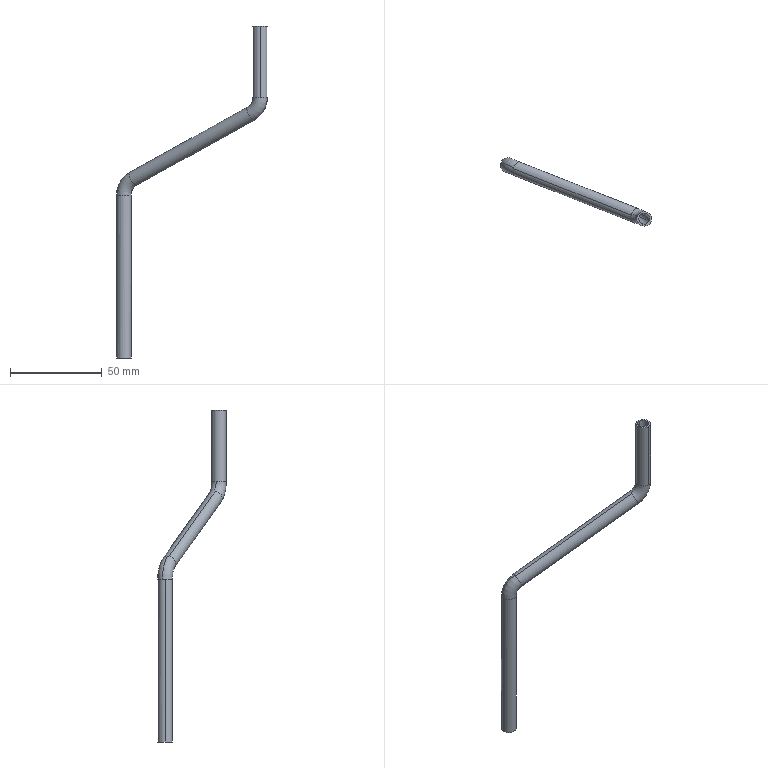Part | NX | features BREP 1 | 1 solid | 22 faces | box 82.41 x 37.379 x 181.231 mm | volume 5003 mm3 | cylinder 12 | torus 8 | plane 2 | commonest cylinder face diameters 6 x6 8 x6
STEP:
#1=CARTESIAN_POINT('',(-2.79,1.102,88.904));
#2=VERTEX_POINT('',#1);
#3=CARTESIAN_POINT('',(-3.,0.,88.904));
#4=VERTEX_POINT('',#3);
#5=CARTESIAN_POINT('',(0.,0.,88.904));
#6=DIRECTION('',(0.,0.,1.));
#7=DIRECTION('',(1.,0.,0.));
#8=AXIS2_PLACEMENT_3D('',#5,#6,#7);
#9=CIRCLE('',#8,3.);
#10=EDGE_CURVE('',#2,#4,#9,.T.);
#11=ORIENTED_EDGE('',*,*,#10,.F.);
#12=CARTESIAN_POINT('',(3.762,-1.485,100.459));
#13=VERTEX_POINT('',#12);
#14=CARTESIAN_POINT('',(9.301,-3.672,88.904));
#15=DIRECTION('',(0.3672,0.9301,0.));
#16=DIRECTION('',(-0.9301,0.3672,0.));
#17=AXIS2_PLACEMENT_3D('',#14,#15,#16);
#18=CIRCLE('',#17,13.);
#19=EDGE_CURVE('',#13,#2,#18,.F.);
#20=ORIENTED_EDGE('',*,*,#19,.F.);
#21=CARTESIAN_POINT('',(3.586,-1.99,100.417));
#22=VERTEX_POINT('',#21);
#23=CARTESIAN_POINT('',(5.04,-1.99,97.793));
#24=DIRECTION('',(0.8268,-0.3264,0.4581));
#25=DIRECTION('',(0.5312,0.1851,-0.8268));
#26=AXIS2_PLACEMENT_3D('',#23,#24,#25);
#27=CIRCLE('',#26,3.);
#28=EDGE_CURVE('',#13,#22,#27,.T.);
#29=ORIENTED_EDGE('',*,*,#28,.T.);
#30=CARTESIAN_POINT('',(6.319,-2.495,95.126));
#31=VERTEX_POINT('',#30);
#32=CARTESIAN_POINT('',(5.04,-1.99,97.793));
#33=DIRECTION('',(0.8268,-0.3264,0.4581));
#34=DIRECTION('',(0.5312,0.1851,-0.8268));
#35=AXIS2_PLACEMENT_3D('',#32,#33,#34);
#36=CIRCLE('',#35,3.);
#37=EDGE_CURVE('',#22,#31,#36,.T.);
#38=ORIENTED_EDGE('',*,*,#37,.T.);
#39=CARTESIAN_POINT('',(2.79,-1.102,88.904));
#40=VERTEX_POINT('',#39);
#41=CARTESIAN_POINT('',(9.301,-3.672,88.904));
#42=DIRECTION('',(0.3672,0.9301,0.));
#43=DIRECTION('',(-0.9301,0.3672,0.));
#44=AXIS2_PLACEMENT_3D('',#41,#42,#43);
#45=CIRCLE('',#44,7.);
#46=EDGE_CURVE('',#31,#40,#45,.F.);
#47=ORIENTED_EDGE('',*,*,#46,.T.);
#48=CARTESIAN_POINT('',(0.,0.,88.904));
#49=DIRECTION('',(0.,0.,1.));
#50=DIRECTION('',(1.,0.,0.));
#51=AXIS2_PLACEMENT_3D('',#48,#49,#50);
#52=CIRCLE('',#51,3.);
#53=EDGE_CURVE('',#4,#40,#52,.T.);
#54=ORIENTED_EDGE('',*,*,#53,.F.);
#55=EDGE_LOOP('',(#11,#20,#29,#38,#47,#54));
#56=FACE_BOUND('',#55,.T.);
#57=CARTESIAN_POINT('',(9.301,-3.672,88.904));
#58=DIRECTION('',(0.3672,0.9301,0.));
#59=DIRECTION('',(-0.9301,0.3672,0.));
#60=AXIS2_PLACEMENT_3D('',#57,#58,#59);
#61=TOROIDAL_SURFACE('',#60,10.,3.);
#62=ADVANCED_FACE('',(#56),#61,.F.);
#63=CARTESIAN_POINT('',(4.,0.,88.904));
#64=VERTEX_POINT('',#63);
#65=CARTESIAN_POINT('',(-3.721,1.469,88.904));
#66=VERTEX_POINT('',#65);
#67=CARTESIAN_POINT('',(0.,0.,88.904));
#68=DIRECTION('',(0.,0.,1.));
#69=DIRECTION('',(1.,0.,0.));
#70=AXIS2_PLACEMENT_3D('',#67,#68,#69);
#71=CIRCLE('',#70,4.);
#72=EDGE_CURVE('',#64,#66,#71,.T.);
#73=ORIENTED_EDGE('',*,*,#72,.T.);
#74=CARTESIAN_POINT('',(3.336,-1.317,101.348));
#75=VERTEX_POINT('',#74);
#76=CARTESIAN_POINT('',(9.301,-3.672,88.904));
#77=DIRECTION('',(0.3672,0.9301,0.));
#78=DIRECTION('',(-0.9301,0.3672,0.));
#79=AXIS2_PLACEMENT_3D('',#76,#77,#78);
#80=CIRCLE('',#79,14.);
#81=EDGE_CURVE('',#75,#66,#80,.F.);
#82=ORIENTED_EDGE('',*,*,#81,.F.);
#83=CARTESIAN_POINT('',(6.979,-1.99,94.294));
#84=VERTEX_POINT('',#83);
#85=CARTESIAN_POINT('',(5.04,-1.99,97.793));
#86=DIRECTION('',(0.8268,-0.3264,0.4581));
#87=DIRECTION('',(0.5312,0.1851,-0.8268));
#88=AXIS2_PLACEMENT_3D('',#85,#86,#87);
#89=CIRCLE('',#88,4.);
#90=EDGE_CURVE('',#84,#75,#89,.T.);
#91=ORIENTED_EDGE('',*,*,#90,.F.);
#92=CARTESIAN_POINT('',(6.745,-2.663,94.237));
#93=VERTEX_POINT('',#92);
#94=CARTESIAN_POINT('',(5.04,-1.99,97.793));
#95=DIRECTION('',(0.8268,-0.3264,0.4581));
#96=DIRECTION('',(0.5312,0.1851,-0.8268));
#97=AXIS2_PLACEMENT_3D('',#94,#95,#96);
#98=CIRCLE('',#97,4.);
#99=EDGE_CURVE('',#93,#84,#98,.T.);
#100=ORIENTED_EDGE('',*,*,#99,.F.);
#101=CARTESIAN_POINT('',(3.721,-1.469,88.904));
#102=VERTEX_POINT('',#101);
#103=CARTESIAN_POINT('',(9.301,-3.672,88.904));
#104=DIRECTION('',(0.3672,0.9301,0.));
#105=DIRECTION('',(-0.9301,0.3672,0.));
#106=AXIS2_PLACEMENT_3D('',#103,#104,#105);
#107=CIRCLE('',#106,6.);
#108=EDGE_CURVE('',#93,#102,#107,.F.);
#109=ORIENTED_EDGE('',*,*,#108,.T.);
#110=CARTESIAN_POINT('',(0.,0.,88.904));
#111=DIRECTION('',(0.,0.,1.));
#112=DIRECTION('',(1.,0.,0.));
#113=AXIS2_PLACEMENT_3D('',#110,#111,#112);
#114=CIRCLE('',#113,4.);
#115=EDGE_CURVE('',#102,#64,#114,.T.);
#116=ORIENTED_EDGE('',*,*,#115,.T.);
#117=EDGE_LOOP('',(#73,#82,#91,#100,#109,#116));
#118=FACE_BOUND('',#117,.T.);
#119=CARTESIAN_POINT('',(9.301,-3.672,88.904));
#120=DIRECTION('',(0.3672,0.9301,0.));
#121=DIRECTION('',(-0.9301,0.3672,0.));
#122=AXIS2_PLACEMENT_3D('',#119,#120,#121);
#123=TOROIDAL_SURFACE('',#122,10.,4.);
#124=ADVANCED_FACE('',(#118),#123,.T.);
#125=CARTESIAN_POINT('',(70.649,-27.893,130.772));
#126=VERTEX_POINT('',#125);
#127=CARTESIAN_POINT('',(70.824,-27.389,130.814));
#128=VERTEX_POINT('',#127);
#129=CARTESIAN_POINT('',(69.37,-27.389,133.438));
#130=DIRECTION('',(0.8268,-0.3264,0.4581));
#131=DIRECTION('',(0.5312,0.1851,-0.8268));
#132=AXIS2_PLACEMENT_3D('',#129,#130,#131);
#133=CIRCLE('',#132,3.);
#134=EDGE_CURVE('',#126,#128,#133,.T.);
#135=ORIENTED_EDGE('',*,*,#134,.F.);
#136=CARTESIAN_POINT('',(77.201,-30.48,142.327));
#137=VERTEX_POINT('',#136);
#138=CARTESIAN_POINT('',(65.109,-25.706,142.327));
#139=DIRECTION('',(-0.3672,-0.9301,0.));
#140=DIRECTION('',(0.9301,-0.3672,0.));
#141=AXIS2_PLACEMENT_3D('',#138,#139,#140);
#142=CIRCLE('',#141,13.);
#143=EDGE_CURVE('',#126,#137,#142,.T.);
#144=ORIENTED_EDGE('',*,*,#143,.T.);
#145=CARTESIAN_POINT('',(74.41,-26.379,142.327));
#146=VERTEX_POINT('',#145);
#147=CARTESIAN_POINT('',(74.41,-29.379,142.327));
#148=DIRECTION('',(0.,0.,1.));
#149=DIRECTION('',(1.,0.,0.));
#150=AXIS2_PLACEMENT_3D('',#147,#148,#149);
#151=CIRCLE('',#150,3.);
#152=EDGE_CURVE('',#137,#146,#151,.T.);
#153=ORIENTED_EDGE('',*,*,#152,.T.);
#154=CARTESIAN_POINT('',(71.62,-28.277,142.327));
#155=VERTEX_POINT('',#154);
#156=CARTESIAN_POINT('',(74.41,-29.379,142.327));
#157=DIRECTION('',(0.,0.,1.));
#158=DIRECTION('',(1.,0.,0.));
#159=AXIS2_PLACEMENT_3D('',#156,#157,#158);
#160=CIRCLE('',#159,3.);
#161=EDGE_CURVE('',#146,#155,#160,.T.);
#162=ORIENTED_EDGE('',*,*,#161,.T.);
#163=CARTESIAN_POINT('',(68.092,-26.884,136.105));
#164=VERTEX_POINT('',#163);
#165=CARTESIAN_POINT('',(65.109,-25.706,142.327));
#166=DIRECTION('',(-0.3672,-0.9301,0.));
#167=DIRECTION('',(0.9301,-0.3672,0.));
#168=AXIS2_PLACEMENT_3D('',#165,#166,#167);
#169=CIRCLE('',#168,7.);
#170=EDGE_CURVE('',#164,#155,#169,.T.);
#171=ORIENTED_EDGE('',*,*,#170,.F.);
#172=CARTESIAN_POINT('',(69.37,-27.389,133.438));
#173=DIRECTION('',(0.8268,-0.3264,0.4581));
#174=DIRECTION('',(0.5312,0.1851,-0.8268));
#175=AXIS2_PLACEMENT_3D('',#172,#173,#174);
#176=CIRCLE('',#175,3.);
#177=EDGE_CURVE('',#128,#164,#176,.T.);
#178=ORIENTED_EDGE('',*,*,#177,.F.);
#179=EDGE_LOOP('',(#135,#144,#153,#162,#171,#178));
#180=FACE_BOUND('',#179,.T.);
#181=CARTESIAN_POINT('',(65.109,-25.706,142.327));
#182=DIRECTION('',(-0.3672,-0.9301,0.));
#183=DIRECTION('',(0.9301,-0.3672,0.));
#184=AXIS2_PLACEMENT_3D('',#181,#182,#183);
#185=TOROIDAL_SURFACE('',#184,10.,3.);
#186=ADVANCED_FACE('',(#180),#185,.F.);
#187=CARTESIAN_POINT('',(67.432,-27.389,136.937));
#188=VERTEX_POINT('',#187);
#189=CARTESIAN_POINT('',(71.075,-28.062,129.883));
#190=VERTEX_POINT('',#189);
#191=CARTESIAN_POINT('',(69.37,-27.389,133.438));
#192=DIRECTION('',(0.8268,-0.3264,0.4581));
#193=DIRECTION('',(0.5312,0.1851,-0.8268));
#194=AXIS2_PLACEMENT_3D('',#191,#192,#193);
#195=CIRCLE('',#194,4.);
#196=EDGE_CURVE('',#188,#190,#195,.T.);
#197=ORIENTED_EDGE('',*,*,#196,.T.);
#198=CARTESIAN_POINT('',(78.131,-30.847,142.327));
#199=VERTEX_POINT('',#198);
#200=CARTESIAN_POINT('',(65.109,-25.706,142.327));
#201=DIRECTION('',(-0.3672,-0.9301,0.));
#202=DIRECTION('',(0.9301,-0.3672,0.));
#203=AXIS2_PLACEMENT_3D('',#200,#201,#202);
#204=CIRCLE('',#203,14.);
#205=EDGE_CURVE('',#190,#199,#204,.T.);
#206=ORIENTED_EDGE('',*,*,#205,.T.);
#207=CARTESIAN_POINT('',(74.41,-33.379,142.327));
#208=VERTEX_POINT('',#207);
#209=CARTESIAN_POINT('',(74.41,-29.379,142.327));
#210=DIRECTION('',(0.,0.,1.));
#211=DIRECTION('',(1.,0.,0.));
#212=AXIS2_PLACEMENT_3D('',#209,#210,#211);
#213=CIRCLE('',#212,4.);
#214=EDGE_CURVE('',#208,#199,#213,.T.);
#215=ORIENTED_EDGE('',*,*,#214,.F.);
#216=CARTESIAN_POINT('',(70.69,-27.91,142.327));
#217=VERTEX_POINT('',#216);
#218=CARTESIAN_POINT('',(74.41,-29.379,142.327));
#219=DIRECTION('',(0.,0.,1.));
#220=DIRECTION('',(1.,0.,0.));
#221=AXIS2_PLACEMENT_3D('',#218,#219,#220);
#222=CIRCLE('',#221,4.);
#223=EDGE_CURVE('',#217,#208,#222,.T.);
#224=ORIENTED_EDGE('',*,*,#223,.F.);
#225=CARTESIAN_POINT('',(67.666,-26.716,136.994));
#226=VERTEX_POINT('',#225);
#227=CARTESIAN_POINT('',(65.109,-25.706,142.327));
#228=DIRECTION('',(-0.3672,-0.9301,0.));
#229=DIRECTION('',(0.9301,-0.3672,0.));
#230=AXIS2_PLACEMENT_3D('',#227,#228,#229);
#231=CIRCLE('',#230,6.);
#232=EDGE_CURVE('',#226,#217,#231,.T.);
#233=ORIENTED_EDGE('',*,*,#232,.F.);
#234=CARTESIAN_POINT('',(69.37,-27.389,133.438));
#235=DIRECTION('',(0.8268,-0.3264,0.4581));
#236=DIRECTION('',(0.5312,0.1851,-0.8268));
#237=AXIS2_PLACEMENT_3D('',#234,#235,#236);
#238=CIRCLE('',#237,4.);
#239=EDGE_CURVE('',#226,#188,#238,.T.);
#240=ORIENTED_EDGE('',*,*,#239,.T.);
#241=EDGE_LOOP('',(#197,#206,#215,#224,#233,#240));
#242=FACE_BOUND('',#241,.T.);
#243=CARTESIAN_POINT('',(65.109,-25.706,142.327));
#244=DIRECTION('',(-0.3672,-0.9301,0.));
#245=DIRECTION('',(0.9301,-0.3672,0.));
#246=AXIS2_PLACEMENT_3D('',#243,#244,#245);
#247=TOROIDAL_SURFACE('',#246,10.,4.);
#248=ADVANCED_FACE('',(#242),#247,.T.);
#249=ORIENTED_EDGE('',*,*,#72,.F.);
#250=CARTESIAN_POINT('',(4.,0.,0.));
#251=VERTEX_POINT('',#250);
#252=CARTESIAN_POINT('',(4.,0.,88.904));
#253=DIRECTION('',(0.,0.,-1.));
#254=VECTOR('',#253,1000.);
#255=LINE('',#252,#254);
#256=EDGE_CURVE('',#64,#251,#255,.T.);
#257=ORIENTED_EDGE('',*,*,#256,.T.);
#258=CARTESIAN_POINT('',(-4.,0.,0.));
#259=VERTEX_POINT('',#258);
#260=CARTESIAN_POINT('',(0.,0.,0.));
#261=DIRECTION('',(0.,0.,1.));
#262=DIRECTION('',(1.,0.,0.));
#263=AXIS2_PLACEMENT_3D('',#260,#261,#262);
#264=CIRCLE('',#263,4.);
#265=EDGE_CURVE('',#251,#259,#264,.T.);
#266=ORIENTED_EDGE('',*,*,#265,.T.);
#267=CARTESIAN_POINT('',(-4.,0.,88.904));
#268=VERTEX_POINT('',#267);
#269=CARTESIAN_POINT('',(-4.,0.,88.904));
#270=DIRECTION('',(0.,0.,-1.));
#271=VECTOR('',#270,1000.);
#272=LINE('',#269,#271);
#273=EDGE_CURVE('',#268,#259,#272,.T.);
#274=ORIENTED_EDGE('',*,*,#273,.F.);
#275=CARTESIAN_POINT('',(0.,0.,88.904));
#276=DIRECTION('',(0.,0.,1.));
#277=DIRECTION('',(1.,0.,0.));
#278=AXIS2_PLACEMENT_3D('',#275,#276,#277);
#279=CIRCLE('',#278,4.);
#280=EDGE_CURVE('',#66,#268,#279,.T.);
#281=ORIENTED_EDGE('',*,*,#280,.F.);
#282=EDGE_LOOP('',(#249,#257,#266,#274,#281));
#283=FACE_BOUND('',#282,.T.);
#284=CARTESIAN_POINT('',(0.,0.,88.904));
#285=DIRECTION('',(0.,0.,-1.));
#286=DIRECTION('',(-1.,0.,0.));
#287=AXIS2_PLACEMENT_3D('',#284,#285,#286);
#288=CYLINDRICAL_SURFACE('',#287,4.);
#289=ADVANCED_FACE('',(#283),#288,.T.);
#290=ORIENTED_EDGE('',*,*,#53,.T.);
#291=CARTESIAN_POINT('',(3.,0.,88.904));
#292=VERTEX_POINT('',#291);
#293=CARTESIAN_POINT('',(0.,0.,88.904));
#294=DIRECTION('',(0.,0.,1.));
#295=DIRECTION('',(1.,0.,0.));
#296=AXIS2_PLACEMENT_3D('',#293,#294,#295);
#297=CIRCLE('',#296,3.);
#298=EDGE_CURVE('',#40,#292,#297,.T.);
#299=ORIENTED_EDGE('',*,*,#298,.T.);
#300=CARTESIAN_POINT('',(3.,0.,0.));
#301=VERTEX_POINT('',#300);
#302=CARTESIAN_POINT('',(3.,0.,88.904));
#303=DIRECTION('',(0.,0.,-1.));
#304=VECTOR('',#303,1000.);
#305=LINE('',#302,#304);
#306=EDGE_CURVE('',#292,#301,#305,.T.);
#307=ORIENTED_EDGE('',*,*,#306,.T.);
#308=CARTESIAN_POINT('',(-3.,0.,0.));
#309=VERTEX_POINT('',#308);
#310=CARTESIAN_POINT('',(0.,0.,0.));
#311=DIRECTION('',(0.,0.,1.));
#312=DIRECTION('',(1.,0.,0.));
#313=AXIS2_PLACEMENT_3D('',#310,#311,#312);
#314=CIRCLE('',#313,3.);
#315=EDGE_CURVE('',#309,#301,#314,.T.);
#316=ORIENTED_EDGE('',*,*,#315,.F.);
#317=CARTESIAN_POINT('',(-3.,0.,88.904));
#318=DIRECTION('',(0.,0.,-1.));
#319=VECTOR('',#318,1000.);
#320=LINE('',#317,#319);
#321=EDGE_CURVE('',#4,#309,#320,.T.);
#322=ORIENTED_EDGE('',*,*,#321,.F.);
#323=EDGE_LOOP('',(#290,#299,#307,#316,#322));
#324=FACE_BOUND('',#323,.T.);
#325=CARTESIAN_POINT('',(0.,0.,88.904));
#326=DIRECTION('',(0.,0.,-1.));
#327=DIRECTION('',(-1.,0.,0.));
#328=AXIS2_PLACEMENT_3D('',#325,#326,#327);
#329=CYLINDRICAL_SURFACE('',#328,3.);
#330=ADVANCED_FACE('',(#324),#329,.F.);
#331=ORIENTED_EDGE('',*,*,#37,.F.);
#332=CARTESIAN_POINT('',(67.916,-27.389,136.062));
#333=VERTEX_POINT('',#332);
#334=CARTESIAN_POINT('',(3.586,-1.99,100.417));
#335=DIRECTION('',(0.8268,-0.3264,0.4581));
#336=VECTOR('',#335,1000.);
#337=LINE('',#334,#336);
#338=EDGE_CURVE('',#333,#22,#337,.F.);
#339=ORIENTED_EDGE('',*,*,#338,.F.);
#340=CARTESIAN_POINT('',(69.37,-27.389,133.438));
#341=DIRECTION('',(0.8268,-0.3264,0.4581));
#342=DIRECTION('',(0.5312,0.1851,-0.8268));
#343=AXIS2_PLACEMENT_3D('',#340,#341,#342);
#344=CIRCLE('',#343,3.);
#345=EDGE_CURVE('',#333,#126,#344,.T.);
#346=ORIENTED_EDGE('',*,*,#345,.T.);
#347=ORIENTED_EDGE('',*,*,#134,.T.);
#348=CARTESIAN_POINT('',(6.494,-1.99,95.169));
#349=VERTEX_POINT('',#348);
#350=CARTESIAN_POINT('',(6.494,-1.99,95.169));
#351=DIRECTION('',(0.8268,-0.3264,0.4581));
#352=VECTOR('',#351,1000.);
#353=LINE('',#350,#352);
#354=EDGE_CURVE('',#128,#349,#353,.F.);
#355=ORIENTED_EDGE('',*,*,#354,.T.);
#356=CARTESIAN_POINT('',(5.04,-1.99,97.793));
#357=DIRECTION('',(0.8268,-0.3264,0.4581));
#358=DIRECTION('',(0.5312,0.1851,-0.8268));
#359=AXIS2_PLACEMENT_3D('',#356,#357,#358);
#360=CIRCLE('',#359,3.);
#361=EDGE_CURVE('',#31,#349,#360,.T.);
#362=ORIENTED_EDGE('',*,*,#361,.F.);
#363=EDGE_LOOP('',(#331,#339,#346,#347,#355,#362));
#364=FACE_BOUND('',#363,.T.);
#365=CARTESIAN_POINT('',(5.04,-1.99,97.793));
#366=DIRECTION('',(0.8268,-0.3264,0.4581));
#367=DIRECTION('',(0.4847,0.,-0.8747));
#368=AXIS2_PLACEMENT_3D('',#365,#366,#367);
#369=CYLINDRICAL_SURFACE('',#368,3.);
#370=ADVANCED_FACE('',(#364),#369,.F.);
#371=ORIENTED_EDGE('',*,*,#90,.T.);
#372=CARTESIAN_POINT('',(3.101,-1.99,101.292));
#373=VERTEX_POINT('',#372);
#374=CARTESIAN_POINT('',(5.04,-1.99,97.793));
#375=DIRECTION('',(0.8268,-0.3264,0.4581));
#376=DIRECTION('',(0.5312,0.1851,-0.8268));
#377=AXIS2_PLACEMENT_3D('',#374,#375,#376);
#378=CIRCLE('',#377,4.);
#379=EDGE_CURVE('',#75,#373,#378,.T.);
#380=ORIENTED_EDGE('',*,*,#379,.T.);
#381=CARTESIAN_POINT('',(3.101,-1.99,101.292));
#382=DIRECTION('',(0.8268,-0.3264,0.4581));
#383=VECTOR('',#382,1000.);
#384=LINE('',#381,#383);
#385=EDGE_CURVE('',#188,#373,#384,.F.);
#386=ORIENTED_EDGE('',*,*,#385,.F.);
#387=ORIENTED_EDGE('',*,*,#239,.F.);
#388=CARTESIAN_POINT('',(71.309,-27.389,129.94));
#389=VERTEX_POINT('',#388);
#390=CARTESIAN_POINT('',(69.37,-27.389,133.438));
#391=DIRECTION('',(0.8268,-0.3264,0.4581));
#392=DIRECTION('',(0.5312,0.1851,-0.8268));
#393=AXIS2_PLACEMENT_3D('',#390,#391,#392);
#394=CIRCLE('',#393,4.);
#395=EDGE_CURVE('',#389,#226,#394,.T.);
#396=ORIENTED_EDGE('',*,*,#395,.F.);
#397=CARTESIAN_POINT('',(6.979,-1.99,94.294));
#398=DIRECTION('',(0.8268,-0.3264,0.4581));
#399=VECTOR('',#398,1000.);
#400=LINE('',#397,#399);
#401=EDGE_CURVE('',#389,#84,#400,.F.);
#402=ORIENTED_EDGE('',*,*,#401,.T.);
#403=EDGE_LOOP('',(#371,#380,#386,#387,#396,#402));
#404=FACE_BOUND('',#403,.T.);
#405=CARTESIAN_POINT('',(5.04,-1.99,97.793));
#406=DIRECTION('',(0.8268,-0.3264,0.4581));
#407=DIRECTION('',(0.4847,0.,-0.8747));
#408=AXIS2_PLACEMENT_3D('',#405,#406,#407);
#409=CYLINDRICAL_SURFACE('',#408,4.);
#410=ADVANCED_FACE('',(#404),#409,.T.);
#411=ORIENTED_EDGE('',*,*,#161,.F.);
#412=CARTESIAN_POINT('',(74.41,-26.379,181.231));
#413=VERTEX_POINT('',#412);
#414=CARTESIAN_POINT('',(74.41,-26.379,142.327));
#415=DIRECTION('',(0.,0.,1.));
#416=VECTOR('',#415,1000.);
#417=LINE('',#414,#416);
#418=EDGE_CURVE('',#146,#413,#417,.T.);
#419=ORIENTED_EDGE('',*,*,#418,.T.);
#420=CARTESIAN_POINT('',(74.41,-32.379,181.231));
#421=VERTEX_POINT('',#420);
#422=CARTESIAN_POINT('',(74.41,-29.379,181.231));
#423=DIRECTION('',(0.,0.,1.));
#424=DIRECTION('',(1.,0.,0.));
#425=AXIS2_PLACEMENT_3D('',#422,#423,#424);
#426=CIRCLE('',#425,3.);
#427=EDGE_CURVE('',#413,#421,#426,.T.);
#428=ORIENTED_EDGE('',*,*,#427,.T.);
#429=CARTESIAN_POINT('',(74.41,-32.379,142.327));
#430=VERTEX_POINT('',#429);
#431=CARTESIAN_POINT('',(74.41,-32.379,142.327));
#432=DIRECTION('',(0.,0.,1.));
#433=VECTOR('',#432,1000.);
#434=LINE('',#431,#433);
#435=EDGE_CURVE('',#430,#421,#434,.T.);
#436=ORIENTED_EDGE('',*,*,#435,.F.);
#437=CARTESIAN_POINT('',(74.41,-29.379,142.327));
#438=DIRECTION('',(0.,0.,1.));
#439=DIRECTION('',(1.,0.,0.));
#440=AXIS2_PLACEMENT_3D('',#437,#438,#439);
#441=CIRCLE('',#440,3.);
#442=EDGE_CURVE('',#155,#430,#441,.T.);
#443=ORIENTED_EDGE('',*,*,#442,.F.);
#444=EDGE_LOOP('',(#411,#419,#428,#436,#443));
#445=FACE_BOUND('',#444,.T.);
#446=CARTESIAN_POINT('',(74.41,-29.379,142.327));
#447=DIRECTION('',(0.,0.,1.));
#448=DIRECTION('',(0.,-1.,0.));
#449=AXIS2_PLACEMENT_3D('',#446,#447,#448);
#450=CYLINDRICAL_SURFACE('',#449,3.);
#451=ADVANCED_FACE('',(#445),#450,.F.);
#452=ORIENTED_EDGE('',*,*,#214,.T.);
#453=CARTESIAN_POINT('',(74.41,-25.379,142.327));
#454=VERTEX_POINT('',#453);
#455=CARTESIAN_POINT('',(74.41,-29.379,142.327));
#456=DIRECTION('',(0.,0.,1.));
#457=DIRECTION('',(1.,0.,0.));
#458=AXIS2_PLACEMENT_3D('',#455,#456,#457);
#459=CIRCLE('',#458,4.);
#460=EDGE_CURVE('',#199,#454,#459,.T.);
#461=ORIENTED_EDGE('',*,*,#460,.T.);
#462=CARTESIAN_POINT('',(74.41,-25.379,181.231));
#463=VERTEX_POINT('',#462);
#464=CARTESIAN_POINT('',(74.41,-25.379,142.327));
#465=DIRECTION('',(0.,0.,1.));
#466=VECTOR('',#465,1000.);
#467=LINE('',#464,#466);
#468=EDGE_CURVE('',#454,#463,#467,.T.);
#469=ORIENTED_EDGE('',*,*,#468,.T.);
#470=CARTESIAN_POINT('',(74.41,-33.379,181.231));
#471=VERTEX_POINT('',#470);
#472=CARTESIAN_POINT('',(74.41,-29.379,181.231));
#473=DIRECTION('',(0.,0.,1.));
#474=DIRECTION('',(1.,0.,0.));
#475=AXIS2_PLACEMENT_3D('',#472,#473,#474);
#476=CIRCLE('',#475,4.);
#477=EDGE_CURVE('',#471,#463,#476,.T.);
#478=ORIENTED_EDGE('',*,*,#477,.F.);
#479=CARTESIAN_POINT('',(74.41,-33.379,142.327));
#480=DIRECTION('',(0.,0.,1.));
#481=VECTOR('',#480,1000.);
#482=LINE('',#479,#481);
#483=EDGE_CURVE('',#208,#471,#482,.T.);
#484=ORIENTED_EDGE('',*,*,#483,.F.);
#485=EDGE_LOOP('',(#452,#461,#469,#478,#484));
#486=FACE_BOUND('',#485,.T.);
#487=CARTESIAN_POINT('',(74.41,-29.379,142.327));
#488=DIRECTION('',(0.,0.,1.));
#489=DIRECTION('',(0.,-1.,0.));
#490=AXIS2_PLACEMENT_3D('',#487,#488,#489);
#491=CYLINDRICAL_SURFACE('',#490,4.);
#492=ADVANCED_FACE('',(#486),#491,.T.);
#493=ORIENTED_EDGE('',*,*,#468,.F.);
#494=CARTESIAN_POINT('',(74.41,-29.379,142.327));
#495=DIRECTION('',(0.,0.,1.));
#496=DIRECTION('',(1.,0.,0.));
#497=AXIS2_PLACEMENT_3D('',#494,#495,#496);
#498=CIRCLE('',#497,4.);
#499=EDGE_CURVE('',#454,#217,#498,.T.);
#500=ORIENTED_EDGE('',*,*,#499,.T.);
#501=ORIENTED_EDGE('',*,*,#223,.T.);
#502=ORIENTED_EDGE('',*,*,#483,.T.);
#503=CARTESIAN_POINT('',(74.41,-29.379,181.231));
#504=DIRECTION('',(0.,0.,1.));
#505=DIRECTION('',(1.,0.,0.));
#506=AXIS2_PLACEMENT_3D('',#503,#504,#505);
#507=CIRCLE('',#506,4.);
#508=EDGE_CURVE('',#463,#471,#507,.T.);
#509=ORIENTED_EDGE('',*,*,#508,.F.);
#510=EDGE_LOOP('',(#493,#500,#501,#502,#509));
#511=FACE_BOUND('',#510,.T.);
#512=CARTESIAN_POINT('',(74.41,-29.379,142.327));
#513=DIRECTION('',(0.,0.,1.));
#514=DIRECTION('',(0.,-1.,0.));
#515=AXIS2_PLACEMENT_3D('',#512,#513,#514);
#516=CYLINDRICAL_SURFACE('',#515,4.);
#517=ADVANCED_FACE('',(#511),#516,.T.);
#518=ORIENTED_EDGE('',*,*,#418,.F.);
#519=ORIENTED_EDGE('',*,*,#152,.F.);
#520=CARTESIAN_POINT('',(74.41,-29.379,142.327));
#521=DIRECTION('',(0.,0.,1.));
#522=DIRECTION('',(1.,0.,0.));
#523=AXIS2_PLACEMENT_3D('',#520,#521,#522);
#524=CIRCLE('',#523,3.);
#525=EDGE_CURVE('',#430,#137,#524,.T.);
#526=ORIENTED_EDGE('',*,*,#525,.F.);
#527=ORIENTED_EDGE('',*,*,#435,.T.);
#528=CARTESIAN_POINT('',(74.41,-29.379,181.231));
#529=DIRECTION('',(0.,0.,1.));
#530=DIRECTION('',(1.,0.,0.));
#531=AXIS2_PLACEMENT_3D('',#528,#529,#530);
#532=CIRCLE('',#531,3.);
#533=EDGE_CURVE('',#421,#413,#532,.T.);
#534=ORIENTED_EDGE('',*,*,#533,.T.);
#535=EDGE_LOOP('',(#518,#519,#526,#527,#534));
#536=FACE_BOUND('',#535,.T.);
#537=CARTESIAN_POINT('',(74.41,-29.379,142.327));
#538=DIRECTION('',(0.,0.,1.));
#539=DIRECTION('',(0.,-1.,0.));
#540=AXIS2_PLACEMENT_3D('',#537,#538,#539);
#541=CYLINDRICAL_SURFACE('',#540,3.);
#542=ADVANCED_FACE('',(#536),#541,.F.);
#543=ORIENTED_EDGE('',*,*,#205,.F.);
#544=CARTESIAN_POINT('',(69.37,-27.389,133.438));
#545=DIRECTION('',(0.8268,-0.3264,0.4581));
#546=DIRECTION('',(0.5312,0.1851,-0.8268));
#547=AXIS2_PLACEMENT_3D('',#544,#545,#546);
#548=CIRCLE('',#547,4.);
#549=EDGE_CURVE('',#190,#389,#548,.T.);
#550=ORIENTED_EDGE('',*,*,#549,.T.);
#551=ORIENTED_EDGE('',*,*,#395,.T.);
#552=ORIENTED_EDGE('',*,*,#232,.T.);
#553=ORIENTED_EDGE('',*,*,#499,.F.);
#554=ORIENTED_EDGE('',*,*,#460,.F.);
#555=EDGE_LOOP('',(#543,#550,#551,#552,#553,#554));
#556=FACE_BOUND('',#555,.T.);
#557=CARTESIAN_POINT('',(65.109,-25.706,142.327));
#558=DIRECTION('',(-0.3672,-0.9301,0.));
#559=DIRECTION('',(0.9301,-0.3672,0.));
#560=AXIS2_PLACEMENT_3D('',#557,#558,#559);
#561=TOROIDAL_SURFACE('',#560,10.,4.);
#562=ADVANCED_FACE('',(#556),#561,.T.);
#563=ORIENTED_EDGE('',*,*,#143,.F.);
#564=ORIENTED_EDGE('',*,*,#345,.F.);
#565=CARTESIAN_POINT('',(69.37,-27.389,133.438));
#566=DIRECTION('',(0.8268,-0.3264,0.4581));
#567=DIRECTION('',(0.5312,0.1851,-0.8268));
#568=AXIS2_PLACEMENT_3D('',#565,#566,#567);
#569=CIRCLE('',#568,3.);
#570=EDGE_CURVE('',#164,#333,#569,.T.);
#571=ORIENTED_EDGE('',*,*,#570,.F.);
#572=ORIENTED_EDGE('',*,*,#170,.T.);
#573=ORIENTED_EDGE('',*,*,#442,.T.);
#574=ORIENTED_EDGE('',*,*,#525,.T.);
#575=EDGE_LOOP('',(#563,#564,#571,#572,#573,#574));
#576=FACE_BOUND('',#575,.T.);
#577=CARTESIAN_POINT('',(65.109,-25.706,142.327));
#578=DIRECTION('',(-0.3672,-0.9301,0.));
#579=DIRECTION('',(0.9301,-0.3672,0.));
#580=AXIS2_PLACEMENT_3D('',#577,#578,#579);
#581=TOROIDAL_SURFACE('',#580,10.,3.);
#582=ADVANCED_FACE('',(#576),#581,.F.);
#583=ORIENTED_EDGE('',*,*,#385,.T.);
#584=CARTESIAN_POINT('',(5.04,-1.99,97.793));
#585=DIRECTION('',(0.8268,-0.3264,0.4581));
#586=DIRECTION('',(0.5312,0.1851,-0.8268));
#587=AXIS2_PLACEMENT_3D('',#584,#585,#586);
#588=CIRCLE('',#587,4.);
#589=EDGE_CURVE('',#373,#93,#588,.T.);
#590=ORIENTED_EDGE('',*,*,#589,.T.);
#591=ORIENTED_EDGE('',*,*,#99,.T.);
#592=ORIENTED_EDGE('',*,*,#401,.F.);
#593=ORIENTED_EDGE('',*,*,#549,.F.);
#594=ORIENTED_EDGE('',*,*,#196,.F.);
#595=EDGE_LOOP('',(#583,#590,#591,#592,#593,#594));
#596=FACE_BOUND('',#595,.T.);
#597=CARTESIAN_POINT('',(5.04,-1.99,97.793));
#598=DIRECTION('',(0.8268,-0.3264,0.4581));
#599=DIRECTION('',(0.4847,0.,-0.8747));
#600=AXIS2_PLACEMENT_3D('',#597,#598,#599);
#601=CYLINDRICAL_SURFACE('',#600,4.);
#602=ADVANCED_FACE('',(#596),#601,.T.);
#603=ORIENTED_EDGE('',*,*,#338,.T.);
#604=ORIENTED_EDGE('',*,*,#28,.F.);
#605=CARTESIAN_POINT('',(5.04,-1.99,97.793));
#606=DIRECTION('',(0.8268,-0.3264,0.4581));
#607=DIRECTION('',(0.5312,0.1851,-0.8268));
#608=AXIS2_PLACEMENT_3D('',#605,#606,#607);
#609=CIRCLE('',#608,3.);
#610=EDGE_CURVE('',#349,#13,#609,.T.);
#611=ORIENTED_EDGE('',*,*,#610,.F.);
#612=ORIENTED_EDGE('',*,*,#354,.F.);
#613=ORIENTED_EDGE('',*,*,#177,.T.);
#614=ORIENTED_EDGE('',*,*,#570,.T.);
#615=EDGE_LOOP('',(#603,#604,#611,#612,#613,#614));
#616=FACE_BOUND('',#615,.T.);
#617=CARTESIAN_POINT('',(5.04,-1.99,97.793));
#618=DIRECTION('',(0.8268,-0.3264,0.4581));
#619=DIRECTION('',(0.4847,0.,-0.8747));
#620=AXIS2_PLACEMENT_3D('',#617,#618,#619);
#621=CYLINDRICAL_SURFACE('',#620,3.);
#622=ADVANCED_FACE('',(#616),#621,.F.);
#623=ORIENTED_EDGE('',*,*,#81,.T.);
#624=ORIENTED_EDGE('',*,*,#280,.T.);
#625=CARTESIAN_POINT('',(0.,0.,88.904));
#626=DIRECTION('',(0.,0.,1.));
#627=DIRECTION('',(1.,0.,0.));
#628=AXIS2_PLACEMENT_3D('',#625,#626,#627);
#629=CIRCLE('',#628,4.);
#630=EDGE_CURVE('',#268,#102,#629,.T.);
#631=ORIENTED_EDGE('',*,*,#630,.T.);
#632=ORIENTED_EDGE('',*,*,#108,.F.);
#633=ORIENTED_EDGE('',*,*,#589,.F.);
#634=ORIENTED_EDGE('',*,*,#379,.F.);
#635=EDGE_LOOP('',(#623,#624,#631,#632,#633,#634));
#636=FACE_BOUND('',#635,.T.);
#637=CARTESIAN_POINT('',(9.301,-3.672,88.904));
#638=DIRECTION('',(0.3672,0.9301,0.));
#639=DIRECTION('',(-0.9301,0.3672,0.));
#640=AXIS2_PLACEMENT_3D('',#637,#638,#639);
#641=TOROIDAL_SURFACE('',#640,10.,4.);
#642=ADVANCED_FACE('',(#636),#641,.T.);
#643=ORIENTED_EDGE('',*,*,#19,.T.);
#644=CARTESIAN_POINT('',(0.,0.,88.904));
#645=DIRECTION('',(0.,0.,1.));
#646=DIRECTION('',(1.,0.,0.));
#647=AXIS2_PLACEMENT_3D('',#644,#645,#646);
#648=CIRCLE('',#647,3.);
#649=EDGE_CURVE('',#292,#2,#648,.T.);
#650=ORIENTED_EDGE('',*,*,#649,.F.);
#651=ORIENTED_EDGE('',*,*,#298,.F.);
#652=ORIENTED_EDGE('',*,*,#46,.F.);
#653=ORIENTED_EDGE('',*,*,#361,.T.);
#654=ORIENTED_EDGE('',*,*,#610,.T.);
#655=EDGE_LOOP('',(#643,#650,#651,#652,#653,#654));
#656=FACE_BOUND('',#655,.T.);
#657=CARTESIAN_POINT('',(9.301,-3.672,88.904));
#658=DIRECTION('',(0.3672,0.9301,0.));
#659=DIRECTION('',(-0.9301,0.3672,0.));
#660=AXIS2_PLACEMENT_3D('',#657,#658,#659);
#661=TOROIDAL_SURFACE('',#660,10.,3.);
#662=ADVANCED_FACE('',(#656),#661,.F.);
#663=ORIENTED_EDGE('',*,*,#306,.F.);
#664=ORIENTED_EDGE('',*,*,#649,.T.);
#665=ORIENTED_EDGE('',*,*,#10,.T.);
#666=ORIENTED_EDGE('',*,*,#321,.T.);
#667=CARTESIAN_POINT('',(0.,0.,0.));
#668=DIRECTION('',(0.,0.,1.));
#669=DIRECTION('',(1.,0.,0.));
#670=AXIS2_PLACEMENT_3D('',#667,#668,#669);
#671=CIRCLE('',#670,3.);
#672=EDGE_CURVE('',#301,#309,#671,.T.);
#673=ORIENTED_EDGE('',*,*,#672,.F.);
#674=EDGE_LOOP('',(#663,#664,#665,#666,#673));
#675=FACE_BOUND('',#674,.T.);
#676=CARTESIAN_POINT('',(0.,0.,88.904));
#677=DIRECTION('',(0.,0.,-1.));
#678=DIRECTION('',(-1.,0.,0.));
#679=AXIS2_PLACEMENT_3D('',#676,#677,#678);
#680=CYLINDRICAL_SURFACE('',#679,3.);
#681=ADVANCED_FACE('',(#675),#680,.F.);
#682=ORIENTED_EDGE('',*,*,#256,.F.);
#683=ORIENTED_EDGE('',*,*,#115,.F.);
#684=ORIENTED_EDGE('',*,*,#630,.F.);
#685=ORIENTED_EDGE('',*,*,#273,.T.);
#686=CARTESIAN_POINT('',(0.,0.,0.));
#687=DIRECTION('',(0.,0.,1.));
#688=DIRECTION('',(1.,0.,0.));
#689=AXIS2_PLACEMENT_3D('',#686,#687,#688);
#690=CIRCLE('',#689,4.);
#691=EDGE_CURVE('',#259,#251,#690,.T.);
#692=ORIENTED_EDGE('',*,*,#691,.T.);
#693=EDGE_LOOP('',(#682,#683,#684,#685,#692));
#694=FACE_BOUND('',#693,.T.);
#695=CARTESIAN_POINT('',(0.,0.,88.904));
#696=DIRECTION('',(0.,0.,-1.));
#697=DIRECTION('',(-1.,0.,0.));
#698=AXIS2_PLACEMENT_3D('',#695,#696,#697);
#699=CYLINDRICAL_SURFACE('',#698,4.);
#700=ADVANCED_FACE('',(#694),#699,.T.);
#701=ORIENTED_EDGE('',*,*,#477,.T.);
#702=ORIENTED_EDGE('',*,*,#508,.T.);
#703=EDGE_LOOP('',(#701,#702));
#704=FACE_BOUND('',#703,.T.);
#705=ORIENTED_EDGE('',*,*,#533,.F.);
#706=ORIENTED_EDGE('',*,*,#427,.F.);
#707=EDGE_LOOP('',(#705,#706));
#708=FACE_BOUND('',#707,.T.);
#709=CARTESIAN_POINT('',(74.41,-29.379,181.231));
#710=DIRECTION('',(0.,0.,1.));
#711=DIRECTION('',(0.,-1.,0.));
#712=AXIS2_PLACEMENT_3D('',#709,#710,#711);
#713=PLANE('',#712);
#714=ADVANCED_FACE('',(#704,#708),#713,.T.);
#715=ORIENTED_EDGE('',*,*,#691,.F.);
#716=ORIENTED_EDGE('',*,*,#265,.F.);
#717=EDGE_LOOP('',(#715,#716));
#718=FACE_BOUND('',#717,.T.);
#719=ORIENTED_EDGE('',*,*,#315,.T.);
#720=ORIENTED_EDGE('',*,*,#672,.T.);
#721=EDGE_LOOP('',(#719,#720));
#722=FACE_BOUND('',#721,.T.);
#723=CARTESIAN_POINT('',(0.,0.,0.));
#724=DIRECTION('',(0.,0.,1.));
#725=DIRECTION('',(1.,0.,0.));
#726=AXIS2_PLACEMENT_3D('',#723,#724,#725);
#727=PLANE('',#726);
#728=ADVANCED_FACE('',(#718,#722),#727,.F.);
#729=CLOSED_SHELL('',(#62,#124,#186,#248,#289,#330,#370,#410,#451,#492,#517,#542,#562,#582,#602,#622,#642,#662,#681,#700,#714,#728));
#730=MANIFOLD_SOLID_BREP('',#729);
#731=(LENGTH_UNIT()NAMED_UNIT(*)SI_UNIT(.MILLI.,.METRE.));
#732=UNCERTAINTY_MEASURE_WITH_UNIT(LENGTH_MEASURE(0.00001),#731,'','');
#733=(NAMED_UNIT(*)PLANE_ANGLE_UNIT()SI_UNIT($,.RADIAN.));
#734=(NAMED_UNIT(*)SI_UNIT($,.STERADIAN.)SOLID_ANGLE_UNIT());
#735=(GEOMETRIC_REPRESENTATION_CONTEXT(3)GLOBAL_UNCERTAINTY_ASSIGNED_CONTEXT((#732))GLOBAL_UNIT_ASSIGNED_CONTEXT((#731,#733,#734))REPRESENTATION_CONTEXT('',''));
#736=ADVANCED_BREP_SHAPE_REPRESENTATION('',(#730),#735);